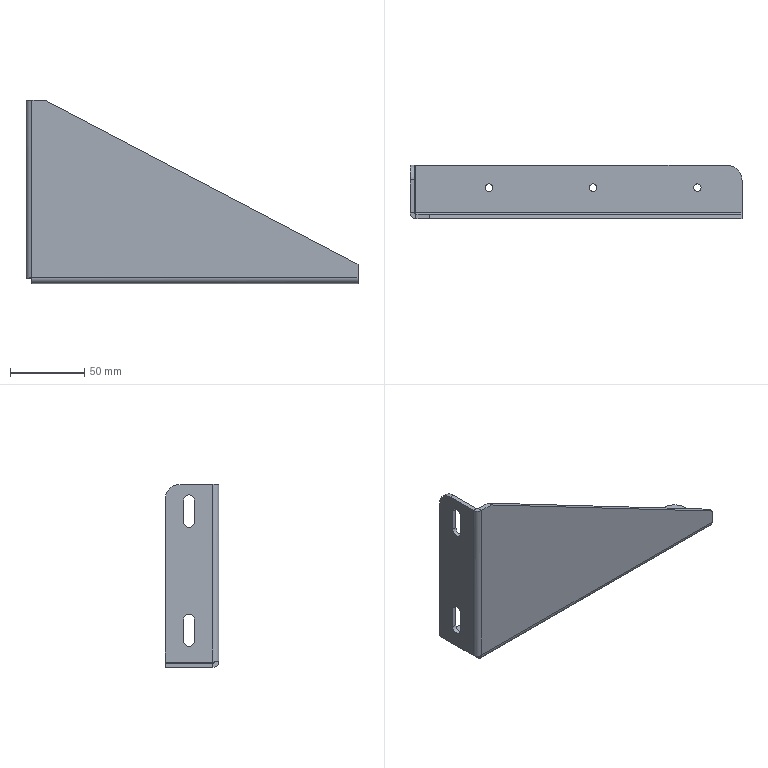Part | SolidWorks | features Cut 1, EdgeFlange 1, Fillet 1, FlatPattern 1, HoleWzd 1, LPattern 1, SMBaseFlange 1, SheetMetal 1 | 1 solid | 39 faces | box 223 x 36 x 123 mm | volume 78856 mm3 | plane 21 | cylinder 16 | spline 2 | commonest cylinder face diameters 5 x6 7 x4 2 x2 8 x2 20 x2
STEP:
#1=CARTESIAN_POINT('',(47.5,21.,-3.));
#2=VERTEX_POINT('',#1);
#3=CARTESIAN_POINT('',(52.5,21.,-3.));
#4=VERTEX_POINT('',#3);
#5=CARTESIAN_POINT('',(50.,21.,-3.));
#6=DIRECTION('',(0.,0.,1.));
#7=DIRECTION('',(1.,0.,0.));
#8=AXIS2_PLACEMENT_3D('',#5,#6,#7);
#9=CIRCLE('',#8,2.5);
#10=EDGE_CURVE('',#2,#4,#9,.T.);
#11=ORIENTED_EDGE('',*,*,#10,.F.);
#12=CARTESIAN_POINT('',(47.5,21.,0.));
#13=VERTEX_POINT('',#12);
#14=CARTESIAN_POINT('',(47.5,21.,0.));
#15=DIRECTION('',(0.,0.,1.));
#16=VECTOR('',#15,1000.);
#17=LINE('',#14,#16);
#18=EDGE_CURVE('',#2,#13,#17,.T.);
#19=ORIENTED_EDGE('',*,*,#18,.T.);
#20=CARTESIAN_POINT('',(52.5,21.,0.));
#21=VERTEX_POINT('',#20);
#22=CARTESIAN_POINT('',(50.,21.,0.));
#23=DIRECTION('',(0.,0.,1.));
#24=DIRECTION('',(1.,0.,0.));
#25=AXIS2_PLACEMENT_3D('',#22,#23,#24);
#26=CIRCLE('',#25,2.5);
#27=EDGE_CURVE('',#13,#21,#26,.T.);
#28=ORIENTED_EDGE('',*,*,#27,.T.);
#29=CARTESIAN_POINT('',(52.5,21.,0.));
#30=DIRECTION('',(0.,0.,1.));
#31=VECTOR('',#30,1000.);
#32=LINE('',#29,#31);
#33=EDGE_CURVE('',#4,#21,#32,.T.);
#34=ORIENTED_EDGE('',*,*,#33,.F.);
#35=EDGE_LOOP('',(#11,#19,#28,#34));
#36=FACE_OUTER_BOUND('',#35,.T.);
#37=CARTESIAN_POINT('',(50.,21.,0.));
#38=DIRECTION('',(0.,0.,1.));
#39=DIRECTION('',(1.,0.,0.));
#40=AXIS2_PLACEMENT_3D('',#37,#38,#39);
#41=CYLINDRICAL_SURFACE('',#40,2.5);
#42=ADVANCED_FACE('',(#36),#41,.F.);
#43=CARTESIAN_POINT('',(117.5,21.,-3.));
#44=VERTEX_POINT('',#43);
#45=CARTESIAN_POINT('',(122.5,21.,-3.));
#46=VERTEX_POINT('',#45);
#47=CARTESIAN_POINT('',(120.,21.,-3.));
#48=DIRECTION('',(0.,0.,1.));
#49=DIRECTION('',(1.,0.,0.));
#50=AXIS2_PLACEMENT_3D('',#47,#48,#49);
#51=CIRCLE('',#50,2.5);
#52=EDGE_CURVE('',#44,#46,#51,.T.);
#53=ORIENTED_EDGE('',*,*,#52,.F.);
#54=CARTESIAN_POINT('',(117.5,21.,0.));
#55=VERTEX_POINT('',#54);
#56=CARTESIAN_POINT('',(117.5,21.,0.));
#57=DIRECTION('',(0.,0.,1.));
#58=VECTOR('',#57,1000.);
#59=LINE('',#56,#58);
#60=EDGE_CURVE('',#44,#55,#59,.T.);
#61=ORIENTED_EDGE('',*,*,#60,.T.);
#62=CARTESIAN_POINT('',(122.5,21.,0.));
#63=VERTEX_POINT('',#62);
#64=CARTESIAN_POINT('',(120.,21.,0.));
#65=DIRECTION('',(0.,0.,1.));
#66=DIRECTION('',(1.,0.,0.));
#67=AXIS2_PLACEMENT_3D('',#64,#65,#66);
#68=CIRCLE('',#67,2.5);
#69=EDGE_CURVE('',#55,#63,#68,.T.);
#70=ORIENTED_EDGE('',*,*,#69,.T.);
#71=CARTESIAN_POINT('',(122.5,21.,0.));
#72=DIRECTION('',(0.,0.,1.));
#73=VECTOR('',#72,1000.);
#74=LINE('',#71,#73);
#75=EDGE_CURVE('',#46,#63,#74,.T.);
#76=ORIENTED_EDGE('',*,*,#75,.F.);
#77=EDGE_LOOP('',(#53,#61,#70,#76));
#78=FACE_OUTER_BOUND('',#77,.T.);
#79=CARTESIAN_POINT('',(120.,21.,0.));
#80=DIRECTION('',(0.,0.,1.));
#81=DIRECTION('',(1.,0.,0.));
#82=AXIS2_PLACEMENT_3D('',#79,#80,#81);
#83=CYLINDRICAL_SURFACE('',#82,2.5);
#84=ADVANCED_FACE('',(#78),#83,.F.);
#85=CARTESIAN_POINT('',(187.5,21.,-3.));
#86=VERTEX_POINT('',#85);
#87=CARTESIAN_POINT('',(192.5,21.,-3.));
#88=VERTEX_POINT('',#87);
#89=CARTESIAN_POINT('',(190.,21.,-3.));
#90=DIRECTION('',(0.,0.,1.));
#91=DIRECTION('',(1.,0.,0.));
#92=AXIS2_PLACEMENT_3D('',#89,#90,#91);
#93=CIRCLE('',#92,2.5);
#94=EDGE_CURVE('',#86,#88,#93,.T.);
#95=ORIENTED_EDGE('',*,*,#94,.F.);
#96=CARTESIAN_POINT('',(187.5,21.,0.));
#97=VERTEX_POINT('',#96);
#98=CARTESIAN_POINT('',(187.5,21.,0.));
#99=DIRECTION('',(0.,0.,1.));
#100=VECTOR('',#99,1000.);
#101=LINE('',#98,#100);
#102=EDGE_CURVE('',#86,#97,#101,.T.);
#103=ORIENTED_EDGE('',*,*,#102,.T.);
#104=CARTESIAN_POINT('',(192.5,21.,0.));
#105=VERTEX_POINT('',#104);
#106=CARTESIAN_POINT('',(190.,21.,0.));
#107=DIRECTION('',(0.,0.,1.));
#108=DIRECTION('',(1.,0.,0.));
#109=AXIS2_PLACEMENT_3D('',#106,#107,#108);
#110=CIRCLE('',#109,2.5);
#111=EDGE_CURVE('',#97,#105,#110,.T.);
#112=ORIENTED_EDGE('',*,*,#111,.T.);
#113=CARTESIAN_POINT('',(192.5,21.,0.));
#114=DIRECTION('',(0.,0.,1.));
#115=VECTOR('',#114,1000.);
#116=LINE('',#113,#115);
#117=EDGE_CURVE('',#88,#105,#116,.T.);
#118=ORIENTED_EDGE('',*,*,#117,.F.);
#119=EDGE_LOOP('',(#95,#103,#112,#118));
#120=FACE_OUTER_BOUND('',#119,.T.);
#121=CARTESIAN_POINT('',(190.,21.,0.));
#122=DIRECTION('',(0.,0.,1.));
#123=DIRECTION('',(1.,0.,0.));
#124=AXIS2_PLACEMENT_3D('',#121,#122,#123);
#125=CYLINDRICAL_SURFACE('',#124,2.5);
#126=ADVANCED_FACE('',(#120),#125,.F.);
#127=CARTESIAN_POINT('',(1.,3.,1.));
#128=VERTEX_POINT('',#127);
#129=CARTESIAN_POINT('',(220.,3.,1.));
#130=VERTEX_POINT('',#129);
#131=CARTESIAN_POINT('',(0.7071,3.,1.));
#132=DIRECTION('',(1.,0.,0.));
#133=VECTOR('',#132,1000.);
#134=LINE('',#131,#133);
#135=EDGE_CURVE('',#128,#130,#134,.T.);
#136=ORIENTED_EDGE('',*,*,#135,.F.);
#137=CARTESIAN_POINT('',(1.,3.,120.));
#138=VERTEX_POINT('',#137);
#139=CARTESIAN_POINT('',(1.,3.,120.));
#140=DIRECTION('',(0.,0.,-1.));
#141=VECTOR('',#140,1000.);
#142=LINE('',#139,#141);
#143=EDGE_CURVE('',#138,#128,#142,.T.);
#144=ORIENTED_EDGE('',*,*,#143,.F.);
#145=CARTESIAN_POINT('',(10.,3.,120.));
#146=VERTEX_POINT('',#145);
#147=CARTESIAN_POINT('',(10.,3.,120.));
#148=DIRECTION('',(1.,0.,0.));
#149=VECTOR('',#148,1000.);
#150=LINE('',#147,#149);
#151=EDGE_CURVE('',#138,#146,#150,.T.);
#152=ORIENTED_EDGE('',*,*,#151,.T.);
#153=CARTESIAN_POINT('',(220.,3.,10.));
#154=VERTEX_POINT('',#153);
#155=CARTESIAN_POINT('',(220.,3.,10.));
#156=DIRECTION('',(0.8858,0.,-0.464));
#157=VECTOR('',#156,1000.);
#158=LINE('',#155,#157);
#159=EDGE_CURVE('',#146,#154,#158,.T.);
#160=ORIENTED_EDGE('',*,*,#159,.T.);
#161=CARTESIAN_POINT('',(220.,3.,0.));
#162=DIRECTION('',(0.,0.,-1.));
#163=VECTOR('',#162,1000.);
#164=LINE('',#161,#163);
#165=EDGE_CURVE('',#154,#130,#164,.T.);
#166=ORIENTED_EDGE('',*,*,#165,.T.);
#167=EDGE_LOOP('',(#136,#144,#152,#160,#166));
#168=FACE_OUTER_BOUND('',#167,.T.);
#169=CARTESIAN_POINT('',(0.,3.,120.));
#170=DIRECTION('',(0.,-1.,0.));
#171=DIRECTION('',(0.,0.,-1.));
#172=AXIS2_PLACEMENT_3D('',#169,#170,#171);
#173=PLANE('',#172);
#174=ADVANCED_FACE('',(#168),#173,.F.);
#175=CARTESIAN_POINT('',(1.,0.,120.));
#176=VERTEX_POINT('',#175);
#177=CARTESIAN_POINT('',(1.,0.,1.));
#178=VERTEX_POINT('',#177);
#179=CARTESIAN_POINT('',(1.,0.,120.));
#180=DIRECTION('',(0.,0.,-1.));
#181=VECTOR('',#180,1000.);
#182=LINE('',#179,#181);
#183=EDGE_CURVE('',#176,#178,#182,.T.);
#184=ORIENTED_EDGE('',*,*,#183,.T.);
#185=CARTESIAN_POINT('',(220.,0.,1.));
#186=VERTEX_POINT('',#185);
#187=CARTESIAN_POINT('',(0.7071,0.,1.));
#188=DIRECTION('',(1.,0.,0.));
#189=VECTOR('',#188,1000.);
#190=LINE('',#187,#189);
#191=EDGE_CURVE('',#178,#186,#190,.T.);
#192=ORIENTED_EDGE('',*,*,#191,.T.);
#193=CARTESIAN_POINT('',(220.,0.,10.));
#194=VERTEX_POINT('',#193);
#195=CARTESIAN_POINT('',(220.,0.,0.));
#196=DIRECTION('',(0.,0.,-1.));
#197=VECTOR('',#196,1000.);
#198=LINE('',#195,#197);
#199=EDGE_CURVE('',#194,#186,#198,.T.);
#200=ORIENTED_EDGE('',*,*,#199,.F.);
#201=CARTESIAN_POINT('',(10.,0.,120.));
#202=VERTEX_POINT('',#201);
#203=CARTESIAN_POINT('',(220.,0.,10.));
#204=DIRECTION('',(0.8858,0.,-0.464));
#205=VECTOR('',#204,1000.);
#206=LINE('',#203,#205);
#207=EDGE_CURVE('',#202,#194,#206,.T.);
#208=ORIENTED_EDGE('',*,*,#207,.F.);
#209=CARTESIAN_POINT('',(10.,0.,120.));
#210=DIRECTION('',(1.,0.,0.));
#211=VECTOR('',#210,1000.);
#212=LINE('',#209,#211);
#213=EDGE_CURVE('',#176,#202,#212,.T.);
#214=ORIENTED_EDGE('',*,*,#213,.F.);
#215=EDGE_LOOP('',(#184,#192,#200,#208,#214));
#216=FACE_OUTER_BOUND('',#215,.T.);
#217=CARTESIAN_POINT('',(0.,0.,120.));
#218=DIRECTION('',(0.,-1.,0.));
#219=DIRECTION('',(0.,0.,-1.));
#220=AXIS2_PLACEMENT_3D('',#217,#218,#219);
#221=PLANE('',#220);
#222=ADVANCED_FACE('',(#216),#221,.T.);
#223=CARTESIAN_POINT('',(220.,3.,1.));
#224=DIRECTION('',(0.,-1.,0.));
#225=VECTOR('',#224,1000.);
#226=LINE('',#223,#225);
#227=EDGE_CURVE('',#130,#186,#226,.T.);
#228=ORIENTED_EDGE('',*,*,#227,.F.);
#229=ORIENTED_EDGE('',*,*,#165,.F.);
#230=CARTESIAN_POINT('',(220.,3.,10.));
#231=DIRECTION('',(0.,-1.,0.));
#232=VECTOR('',#231,1000.);
#233=LINE('',#230,#232);
#234=EDGE_CURVE('',#154,#194,#233,.T.);
#235=ORIENTED_EDGE('',*,*,#234,.T.);
#236=ORIENTED_EDGE('',*,*,#199,.T.);
#237=EDGE_LOOP('',(#228,#229,#235,#236));
#238=FACE_OUTER_BOUND('',#237,.T.);
#239=CARTESIAN_POINT('',(220.,3.,0.));
#240=DIRECTION('',(-1.,0.,0.));
#241=DIRECTION('',(0.,0.,1.));
#242=AXIS2_PLACEMENT_3D('',#239,#240,#241);
#243=PLANE('',#242);
#244=ADVANCED_FACE('',(#238),#243,.F.);
#245=CARTESIAN_POINT('',(1.,3.,120.));
#246=DIRECTION('',(0.,-1.,0.));
#247=VECTOR('',#246,1000.);
#248=LINE('',#245,#247);
#249=EDGE_CURVE('',#138,#176,#248,.T.);
#250=ORIENTED_EDGE('',*,*,#249,.T.);
#251=ORIENTED_EDGE('',*,*,#213,.T.);
#252=CARTESIAN_POINT('',(10.,3.,120.));
#253=DIRECTION('',(0.,-1.,0.));
#254=VECTOR('',#253,1000.);
#255=LINE('',#252,#254);
#256=EDGE_CURVE('',#146,#202,#255,.T.);
#257=ORIENTED_EDGE('',*,*,#256,.F.);
#258=ORIENTED_EDGE('',*,*,#151,.F.);
#259=EDGE_LOOP('',(#250,#251,#257,#258));
#260=FACE_OUTER_BOUND('',#259,.T.);
#261=CARTESIAN_POINT('',(10.,3.,120.));
#262=DIRECTION('',(0.,0.,-1.));
#263=DIRECTION('',(-1.,0.,0.));
#264=AXIS2_PLACEMENT_3D('',#261,#262,#263);
#265=PLANE('',#264);
#266=ADVANCED_FACE('',(#260),#265,.F.);
#267=ORIENTED_EDGE('',*,*,#207,.T.);
#268=ORIENTED_EDGE('',*,*,#234,.F.);
#269=ORIENTED_EDGE('',*,*,#159,.F.);
#270=ORIENTED_EDGE('',*,*,#256,.T.);
#271=EDGE_LOOP('',(#267,#268,#269,#270));
#272=FACE_OUTER_BOUND('',#271,.T.);
#273=CARTESIAN_POINT('',(220.,3.,10.));
#274=DIRECTION('',(-0.464,0.,-0.8858));
#275=DIRECTION('',(-0.8858,0.,0.464));
#276=AXIS2_PLACEMENT_3D('',#273,#274,#275);
#277=PLANE('',#276);
#278=ADVANCED_FACE('',(#272),#277,.F.);
#279=CARTESIAN_POINT('',(-3.,4.,0.7071));
#280=VERTEX_POINT('',#279);
#281=CARTESIAN_POINT('',(0.,4.,0.7071));
#282=VERTEX_POINT('',#281);
#283=CARTESIAN_POINT('',(0.,4.,0.7071));
#284=DIRECTION('',(1.,0.,0.));
#285=VECTOR('',#284,1000.);
#286=LINE('',#283,#285);
#287=EDGE_CURVE('',#280,#282,#286,.T.);
#288=ORIENTED_EDGE('',*,*,#287,.T.);
#289=CARTESIAN_POINT('',(1.,3.,1.));
#290=CARTESIAN_POINT('',(0.7382,3.,0.9512));
#291=CARTESIAN_POINT('',(0.478,3.108,0.9024));
#292=CARTESIAN_POINT('',(0.1078,3.478,0.8047));
#293=CARTESIAN_POINT('',(0.,3.738,0.7559));
#294=CARTESIAN_POINT('',(0.,4.,0.7071));
#295=B_SPLINE_CURVE_WITH_KNOTS('',3,(#289,#290,#291,#292,#293,#294),.UNSPECIFIED.,.F.,.F.,(4,2,4),(0.,0.5,1.),.UNSPECIFIED.);
#296=EDGE_CURVE('',#128,#282,#295,.T.);
#297=ORIENTED_EDGE('',*,*,#296,.F.);
#298=CARTESIAN_POINT('',(1.,3.,1.));
#299=DIRECTION('',(0.,-1.,0.));
#300=VECTOR('',#299,1000.);
#301=LINE('',#298,#300);
#302=EDGE_CURVE('',#128,#178,#301,.T.);
#303=ORIENTED_EDGE('',*,*,#302,.T.);
#304=CARTESIAN_POINT('',(1.,0.,1.));
#305=CARTESIAN_POINT('',(0.4764,0.,0.9756));
#306=CARTESIAN_POINT('',(-0.04699,0.1041,0.9512));
#307=CARTESIAN_POINT('',(-1.014,0.5049,0.9024));
#308=CARTESIAN_POINT('',(-1.458,0.8013,0.878));
#309=CARTESIAN_POINT('',(-2.199,1.542,0.8291));
#310=CARTESIAN_POINT('',(-2.495,1.986,0.8047));
#311=CARTESIAN_POINT('',(-2.896,2.953,0.7559));
#312=CARTESIAN_POINT('',(-3.,3.476,0.7315));
#313=CARTESIAN_POINT('',(-3.,4.,0.7071));
#314=B_SPLINE_CURVE_WITH_KNOTS('',3,(#304,#305,#306,#307,#308,#309,#310,#311,#312,#313),.UNSPECIFIED.,.F.,.F.,(4,2,2,2,4),(0.,0.25,0.5,0.75,1.),.UNSPECIFIED.);
#315=EDGE_CURVE('',#178,#280,#314,.T.);
#316=ORIENTED_EDGE('',*,*,#315,.T.);
#317=EDGE_LOOP('',(#288,#297,#303,#316));
#318=FACE_OUTER_BOUND('',#317,.T.);
#319=CARTESIAN_POINT('',(1.,-0.03,1.));
#320=CARTESIAN_POINT('',(0.4724,-0.03,0.9756));
#321=CARTESIAN_POINT('',(-0.05484,0.07489,0.9512));
#322=CARTESIAN_POINT('',(-1.03,0.4786,0.9024));
#323=CARTESIAN_POINT('',(-1.477,0.7773,0.878));
#324=CARTESIAN_POINT('',(-2.223,1.523,0.8291));
#325=CARTESIAN_POINT('',(-2.521,1.97,0.8047));
#326=CARTESIAN_POINT('',(-2.925,2.945,0.7559));
#327=CARTESIAN_POINT('',(-3.03,3.472,0.7315));
#328=CARTESIAN_POINT('',(-3.03,4.,0.7071));
#329=CARTESIAN_POINT('',(1.,0.,1.));
#330=CARTESIAN_POINT('',(0.4763,0.,0.9756));
#331=CARTESIAN_POINT('',(-0.04699,0.1041,0.9512));
#332=CARTESIAN_POINT('',(-1.014,0.5049,0.9024));
#333=CARTESIAN_POINT('',(-1.458,0.8013,0.878));
#334=CARTESIAN_POINT('',(-2.199,1.542,0.8291));
#335=CARTESIAN_POINT('',(-2.495,1.986,0.8047));
#336=CARTESIAN_POINT('',(-2.896,2.953,0.7559));
#337=CARTESIAN_POINT('',(-3.,3.476,0.7315));
#338=CARTESIAN_POINT('',(-3.,4.,0.7071));
#339=CARTESIAN_POINT('',(1.,3.,1.));
#340=CARTESIAN_POINT('',(0.8691,3.,0.9756));
#341=CARTESIAN_POINT('',(0.7383,3.026,0.9512));
#342=CARTESIAN_POINT('',(0.4964,3.126,0.9024));
#343=CARTESIAN_POINT('',(0.3855,3.2,0.878));
#344=CARTESIAN_POINT('',(0.2003,3.385,0.8291));
#345=CARTESIAN_POINT('',(0.1262,3.496,0.8047));
#346=CARTESIAN_POINT('',(0.02603,3.738,0.7559));
#347=CARTESIAN_POINT('',(0.,3.869,0.7315));
#348=CARTESIAN_POINT('',(0.,4.,0.7071));
#349=CARTESIAN_POINT('',(1.,3.03,1.));
#350=CARTESIAN_POINT('',(0.873,3.03,0.9756));
#351=CARTESIAN_POINT('',(0.7462,3.056,0.9512));
#352=CARTESIAN_POINT('',(0.5116,3.153,0.9024));
#353=CARTESIAN_POINT('',(0.4041,3.225,0.878));
#354=CARTESIAN_POINT('',(0.2246,3.404,0.8291));
#355=CARTESIAN_POINT('',(0.1527,3.512,0.8047));
#356=CARTESIAN_POINT('',(0.05554,3.746,0.7559));
#357=CARTESIAN_POINT('',(0.0303,3.873,0.7315));
#358=CARTESIAN_POINT('',(0.0303,4.,0.7071));
#359=B_SPLINE_SURFACE_WITH_KNOTS('',1,3,((#319,#320,#321,#322,#323,#324,#325,#326,#327,#328),(#329,#330,#331,#332,#333,#334,#335,#336,#337,#338),(#339,#340,#341,#342,#343,#344,#345,#346,#347,#348),(#349,#350,#351,#352,#353,#354,#355,#356,#357,#358)),.UNSPECIFIED.,.F.,.F.,.F.,(2,1,1,2),(4,2,2,2,4),(-0.01,0.,1.,1.01),(0.,0.25,0.5,0.75,1.),.UNSPECIFIED.);
#360=ADVANCED_FACE('',(#318),#359,.F.);
#361=ORIENTED_EDGE('',*,*,#183,.F.);
#362=CARTESIAN_POINT('',(-3.,4.,120.));
#363=VERTEX_POINT('',#362);
#364=CARTESIAN_POINT('',(1.,4.,120.));
#365=DIRECTION('',(0.,0.,1.));
#366=DIRECTION('',(1.,0.,0.));
#367=AXIS2_PLACEMENT_3D('',#364,#365,#366);
#368=CIRCLE('',#367,4.);
#369=EDGE_CURVE('',#363,#176,#368,.T.);
#370=ORIENTED_EDGE('',*,*,#369,.F.);
#371=CARTESIAN_POINT('',(-3.,4.,0.));
#372=DIRECTION('',(0.,0.,-1.));
#373=VECTOR('',#372,1000.);
#374=LINE('',#371,#373);
#375=EDGE_CURVE('',#363,#280,#374,.T.);
#376=ORIENTED_EDGE('',*,*,#375,.T.);
#377=ORIENTED_EDGE('',*,*,#315,.F.);
#378=EDGE_LOOP('',(#361,#370,#376,#377));
#379=FACE_OUTER_BOUND('',#378,.T.);
#380=CARTESIAN_POINT('',(1.,4.,120.));
#381=DIRECTION('',(0.,0.,1.));
#382=DIRECTION('',(-1.,0.,0.));
#383=AXIS2_PLACEMENT_3D('',#380,#381,#382);
#384=CYLINDRICAL_SURFACE('',#383,4.);
#385=ADVANCED_FACE('',(#379),#384,.T.);
#386=CARTESIAN_POINT('',(0.,4.,120.));
#387=VERTEX_POINT('',#386);
#388=CARTESIAN_POINT('',(1.,4.,120.));
#389=DIRECTION('',(0.,0.,1.));
#390=DIRECTION('',(1.,0.,0.));
#391=AXIS2_PLACEMENT_3D('',#388,#389,#390);
#392=CIRCLE('',#391,1.);
#393=EDGE_CURVE('',#387,#138,#392,.T.);
#394=ORIENTED_EDGE('',*,*,#393,.F.);
#395=CARTESIAN_POINT('',(0.,4.,120.));
#396=DIRECTION('',(-1.,0.,0.));
#397=VECTOR('',#396,1000.);
#398=LINE('',#395,#397);
#399=EDGE_CURVE('',#387,#363,#398,.T.);
#400=ORIENTED_EDGE('',*,*,#399,.T.);
#401=ORIENTED_EDGE('',*,*,#369,.T.);
#402=ORIENTED_EDGE('',*,*,#249,.F.);
#403=EDGE_LOOP('',(#394,#400,#401,#402));
#404=FACE_OUTER_BOUND('',#403,.T.);
#405=CARTESIAN_POINT('',(1.,4.,120.));
#406=DIRECTION('',(0.,0.,-1.));
#407=DIRECTION('',(-1.,0.,0.));
#408=AXIS2_PLACEMENT_3D('',#405,#406,#407);
#409=PLANE('',#408);
#410=ADVANCED_FACE('',(#404),#409,.F.);
#411=ORIENTED_EDGE('',*,*,#143,.T.);
#412=ORIENTED_EDGE('',*,*,#296,.T.);
#413=CARTESIAN_POINT('',(0.,4.,0.));
#414=DIRECTION('',(0.,0.,1.));
#415=VECTOR('',#414,1000.);
#416=LINE('',#413,#415);
#417=EDGE_CURVE('',#282,#387,#416,.T.);
#418=ORIENTED_EDGE('',*,*,#417,.T.);
#419=ORIENTED_EDGE('',*,*,#393,.T.);
#420=EDGE_LOOP('',(#411,#412,#418,#419));
#421=FACE_OUTER_BOUND('',#420,.T.);
#422=CARTESIAN_POINT('',(1.,4.,120.));
#423=DIRECTION('',(0.,0.,1.));
#424=DIRECTION('',(-1.,0.,0.));
#425=AXIS2_PLACEMENT_3D('',#422,#423,#424);
#426=CYLINDRICAL_SURFACE('',#425,1.);
#427=ADVANCED_FACE('',(#421),#426,.F.);
#428=CARTESIAN_POINT('',(-3.,36.,0.7071));
#429=VERTEX_POINT('',#428);
#430=CARTESIAN_POINT('',(-3.,36.,0.7071));
#431=DIRECTION('',(0.,1.,0.));
#432=VECTOR('',#431,1000.);
#433=LINE('',#430,#432);
#434=EDGE_CURVE('',#280,#429,#433,.T.);
#435=ORIENTED_EDGE('',*,*,#434,.T.);
#436=CARTESIAN_POINT('',(0.,36.,0.7071));
#437=VERTEX_POINT('',#436);
#438=CARTESIAN_POINT('',(-3.,36.,0.7071));
#439=DIRECTION('',(1.,0.,0.));
#440=VECTOR('',#439,1000.);
#441=LINE('',#438,#440);
#442=EDGE_CURVE('',#429,#437,#441,.T.);
#443=ORIENTED_EDGE('',*,*,#442,.T.);
#444=CARTESIAN_POINT('',(0.,3.,0.7071));
#445=DIRECTION('',(0.,1.,0.));
#446=VECTOR('',#445,1000.);
#447=LINE('',#444,#446);
#448=EDGE_CURVE('',#282,#437,#447,.T.);
#449=ORIENTED_EDGE('',*,*,#448,.F.);
#450=ORIENTED_EDGE('',*,*,#287,.F.);
#451=EDGE_LOOP('',(#435,#443,#449,#450));
#452=FACE_OUTER_BOUND('',#451,.T.);
#453=CARTESIAN_POINT('',(0.,3.,0.7071));
#454=DIRECTION('',(0.,0.,-1.));
#455=DIRECTION('',(-1.,0.,0.));
#456=AXIS2_PLACEMENT_3D('',#453,#454,#455);
#457=PLANE('',#456);
#458=ADVANCED_FACE('',(#452),#457,.T.);
#459=CARTESIAN_POINT('',(-3.,23.5,14.5));
#460=VERTEX_POINT('',#459);
#461=CARTESIAN_POINT('',(-3.,23.5,29.5));
#462=VERTEX_POINT('',#461);
#463=CARTESIAN_POINT('',(-3.,23.5,0.));
#464=DIRECTION('',(0.,0.,1.));
#465=VECTOR('',#464,1000.);
#466=LINE('',#463,#465);
#467=EDGE_CURVE('',#460,#462,#466,.T.);
#468=ORIENTED_EDGE('',*,*,#467,.T.);
#469=CARTESIAN_POINT('',(-3.,16.5,29.5));
#470=VERTEX_POINT('',#469);
#471=CARTESIAN_POINT('',(-3.,20.,29.5));
#472=DIRECTION('',(1.,0.,0.));
#473=DIRECTION('',(0.,1.,0.));
#474=AXIS2_PLACEMENT_3D('',#471,#472,#473);
#475=CIRCLE('',#474,3.5);
#476=EDGE_CURVE('',#462,#470,#475,.T.);
#477=ORIENTED_EDGE('',*,*,#476,.T.);
#478=CARTESIAN_POINT('',(-3.,16.5,14.5));
#479=VERTEX_POINT('',#478);
#480=CARTESIAN_POINT('',(-3.,16.5,0.));
#481=DIRECTION('',(0.,0.,-1.));
#482=VECTOR('',#481,1000.);
#483=LINE('',#480,#482);
#484=EDGE_CURVE('',#470,#479,#483,.T.);
#485=ORIENTED_EDGE('',*,*,#484,.T.);
#486=CARTESIAN_POINT('',(-3.,20.,14.5));
#487=DIRECTION('',(1.,0.,0.));
#488=DIRECTION('',(0.,1.,0.));
#489=AXIS2_PLACEMENT_3D('',#486,#487,#488);
#490=CIRCLE('',#489,3.5);
#491=EDGE_CURVE('',#479,#460,#490,.T.);
#492=ORIENTED_EDGE('',*,*,#491,.T.);
#493=EDGE_LOOP('',(#468,#477,#485,#492));
#494=FACE_BOUND('',#493,.T.);
#495=CARTESIAN_POINT('',(-3.,23.5,94.5));
#496=VERTEX_POINT('',#495);
#497=CARTESIAN_POINT('',(-3.,23.5,109.5));
#498=VERTEX_POINT('',#497);
#499=CARTESIAN_POINT('',(-3.,23.5,0.));
#500=DIRECTION('',(0.,0.,1.));
#501=VECTOR('',#500,1000.);
#502=LINE('',#499,#501);
#503=EDGE_CURVE('',#496,#498,#502,.T.);
#504=ORIENTED_EDGE('',*,*,#503,.T.);
#505=CARTESIAN_POINT('',(-3.,16.5,109.5));
#506=VERTEX_POINT('',#505);
#507=CARTESIAN_POINT('',(-3.,20.,109.5));
#508=DIRECTION('',(1.,0.,0.));
#509=DIRECTION('',(0.,1.,0.));
#510=AXIS2_PLACEMENT_3D('',#507,#508,#509);
#511=CIRCLE('',#510,3.5);
#512=EDGE_CURVE('',#498,#506,#511,.T.);
#513=ORIENTED_EDGE('',*,*,#512,.T.);
#514=CARTESIAN_POINT('',(-3.,16.5,94.5));
#515=VERTEX_POINT('',#514);
#516=CARTESIAN_POINT('',(-3.,16.5,0.));
#517=DIRECTION('',(0.,0.,-1.));
#518=VECTOR('',#517,1000.);
#519=LINE('',#516,#518);
#520=EDGE_CURVE('',#506,#515,#519,.T.);
#521=ORIENTED_EDGE('',*,*,#520,.T.);
#522=CARTESIAN_POINT('',(-3.,20.,94.5));
#523=DIRECTION('',(1.,0.,0.));
#524=DIRECTION('',(0.,1.,0.));
#525=AXIS2_PLACEMENT_3D('',#522,#523,#524);
#526=CIRCLE('',#525,3.5);
#527=EDGE_CURVE('',#515,#496,#526,.T.);
#528=ORIENTED_EDGE('',*,*,#527,.T.);
#529=EDGE_LOOP('',(#504,#513,#521,#528));
#530=FACE_BOUND('',#529,.T.);
#531=CARTESIAN_POINT('',(-3.,26.,120.));
#532=VERTEX_POINT('',#531);
#533=CARTESIAN_POINT('',(-3.,36.,120.));
#534=DIRECTION('',(0.,1.,0.));
#535=VECTOR('',#534,1000.);
#536=LINE('',#533,#535);
#537=EDGE_CURVE('',#363,#532,#536,.T.);
#538=ORIENTED_EDGE('',*,*,#537,.T.);
#539=CARTESIAN_POINT('',(-3.,36.,110.));
#540=VERTEX_POINT('',#539);
#541=CARTESIAN_POINT('',(-3.,26.,110.));
#542=DIRECTION('',(-1.,0.,0.));
#543=DIRECTION('',(0.,1.,0.));
#544=AXIS2_PLACEMENT_3D('',#541,#542,#543);
#545=CIRCLE('',#544,10.);
#546=EDGE_CURVE('',#532,#540,#545,.T.);
#547=ORIENTED_EDGE('',*,*,#546,.T.);
#548=CARTESIAN_POINT('',(-3.,36.,0.));
#549=DIRECTION('',(0.,0.,-1.));
#550=VECTOR('',#549,1000.);
#551=LINE('',#548,#550);
#552=EDGE_CURVE('',#540,#429,#551,.T.);
#553=ORIENTED_EDGE('',*,*,#552,.T.);
#554=ORIENTED_EDGE('',*,*,#434,.F.);
#555=ORIENTED_EDGE('',*,*,#375,.F.);
#556=EDGE_LOOP('',(#538,#547,#553,#554,#555));
#557=FACE_OUTER_BOUND('',#556,.T.);
#558=CARTESIAN_POINT('',(-3.,36.,0.));
#559=DIRECTION('',(1.,0.,0.));
#560=DIRECTION('',(0.,1.,0.));
#561=AXIS2_PLACEMENT_3D('',#558,#559,#560);
#562=PLANE('',#561);
#563=ADVANCED_FACE('',(#494,#530,#557),#562,.F.);
#564=CARTESIAN_POINT('',(0.,23.5,29.5));
#565=VERTEX_POINT('',#564);
#566=CARTESIAN_POINT('',(0.,16.5,29.5));
#567=VERTEX_POINT('',#566);
#568=CARTESIAN_POINT('',(0.,20.,29.5));
#569=DIRECTION('',(1.,0.,0.));
#570=DIRECTION('',(0.,1.,0.));
#571=AXIS2_PLACEMENT_3D('',#568,#569,#570);
#572=CIRCLE('',#571,3.5);
#573=EDGE_CURVE('',#565,#567,#572,.T.);
#574=ORIENTED_EDGE('',*,*,#573,.F.);
#575=CARTESIAN_POINT('',(0.,23.5,14.5));
#576=VERTEX_POINT('',#575);
#577=CARTESIAN_POINT('',(0.,23.5,29.5));
#578=DIRECTION('',(0.,0.,1.));
#579=VECTOR('',#578,1000.);
#580=LINE('',#577,#579);
#581=EDGE_CURVE('',#576,#565,#580,.T.);
#582=ORIENTED_EDGE('',*,*,#581,.F.);
#583=CARTESIAN_POINT('',(0.,16.5,14.5));
#584=VERTEX_POINT('',#583);
#585=CARTESIAN_POINT('',(0.,20.,14.5));
#586=DIRECTION('',(1.,0.,0.));
#587=DIRECTION('',(0.,-1.,0.));
#588=AXIS2_PLACEMENT_3D('',#585,#586,#587);
#589=CIRCLE('',#588,3.5);
#590=EDGE_CURVE('',#584,#576,#589,.T.);
#591=ORIENTED_EDGE('',*,*,#590,.F.);
#592=CARTESIAN_POINT('',(0.,16.5,29.5));
#593=DIRECTION('',(0.,0.,-1.));
#594=VECTOR('',#593,1000.);
#595=LINE('',#592,#594);
#596=EDGE_CURVE('',#567,#584,#595,.T.);
#597=ORIENTED_EDGE('',*,*,#596,.F.);
#598=EDGE_LOOP('',(#574,#582,#591,#597));
#599=FACE_BOUND('',#598,.T.);
#600=CARTESIAN_POINT('',(0.,23.5,109.5));
#601=VERTEX_POINT('',#600);
#602=CARTESIAN_POINT('',(0.,16.5,109.5));
#603=VERTEX_POINT('',#602);
#604=CARTESIAN_POINT('',(0.,20.,109.5));
#605=DIRECTION('',(1.,0.,0.));
#606=DIRECTION('',(0.,1.,0.));
#607=AXIS2_PLACEMENT_3D('',#604,#605,#606);
#608=CIRCLE('',#607,3.5);
#609=EDGE_CURVE('',#601,#603,#608,.T.);
#610=ORIENTED_EDGE('',*,*,#609,.F.);
#611=CARTESIAN_POINT('',(0.,23.5,94.5));
#612=VERTEX_POINT('',#611);
#613=CARTESIAN_POINT('',(0.,23.5,109.5));
#614=DIRECTION('',(0.,0.,1.));
#615=VECTOR('',#614,1000.);
#616=LINE('',#613,#615);
#617=EDGE_CURVE('',#612,#601,#616,.T.);
#618=ORIENTED_EDGE('',*,*,#617,.F.);
#619=CARTESIAN_POINT('',(0.,16.5,94.5));
#620=VERTEX_POINT('',#619);
#621=CARTESIAN_POINT('',(0.,20.,94.5));
#622=DIRECTION('',(1.,0.,0.));
#623=DIRECTION('',(0.,-1.,0.));
#624=AXIS2_PLACEMENT_3D('',#621,#622,#623);
#625=CIRCLE('',#624,3.5);
#626=EDGE_CURVE('',#620,#612,#625,.T.);
#627=ORIENTED_EDGE('',*,*,#626,.F.);
#628=CARTESIAN_POINT('',(0.,16.5,109.5));
#629=DIRECTION('',(0.,0.,-1.));
#630=VECTOR('',#629,1000.);
#631=LINE('',#628,#630);
#632=EDGE_CURVE('',#603,#620,#631,.T.);
#633=ORIENTED_EDGE('',*,*,#632,.F.);
#634=EDGE_LOOP('',(#610,#618,#627,#633));
#635=FACE_BOUND('',#634,.T.);
#636=CARTESIAN_POINT('',(0.,36.,110.));
#637=VERTEX_POINT('',#636);
#638=CARTESIAN_POINT('',(0.,36.,0.));
#639=DIRECTION('',(0.,0.,-1.));
#640=VECTOR('',#639,1000.);
#641=LINE('',#638,#640);
#642=EDGE_CURVE('',#637,#437,#641,.T.);
#643=ORIENTED_EDGE('',*,*,#642,.F.);
#644=CARTESIAN_POINT('',(0.,26.,120.));
#645=VERTEX_POINT('',#644);
#646=CARTESIAN_POINT('',(0.,26.,110.));
#647=DIRECTION('',(1.,0.,0.));
#648=DIRECTION('',(0.,1.,0.));
#649=AXIS2_PLACEMENT_3D('',#646,#647,#648);
#650=CIRCLE('',#649,10.);
#651=EDGE_CURVE('',#637,#645,#650,.T.);
#652=ORIENTED_EDGE('',*,*,#651,.T.);
#653=CARTESIAN_POINT('',(0.,36.,120.));
#654=DIRECTION('',(0.,1.,0.));
#655=VECTOR('',#654,1000.);
#656=LINE('',#653,#655);
#657=EDGE_CURVE('',#387,#645,#656,.T.);
#658=ORIENTED_EDGE('',*,*,#657,.F.);
#659=ORIENTED_EDGE('',*,*,#417,.F.);
#660=ORIENTED_EDGE('',*,*,#448,.T.);
#661=EDGE_LOOP('',(#643,#652,#658,#659,#660));
#662=FACE_OUTER_BOUND('',#661,.T.);
#663=CARTESIAN_POINT('',(0.,36.,0.));
#664=DIRECTION('',(1.,0.,0.));
#665=DIRECTION('',(0.,1.,0.));
#666=AXIS2_PLACEMENT_3D('',#663,#664,#665);
#667=PLANE('',#666);
#668=ADVANCED_FACE('',(#599,#635,#662),#667,.T.);
#669=ORIENTED_EDGE('',*,*,#552,.F.);
#670=CARTESIAN_POINT('',(-3.,36.,110.));
#671=DIRECTION('',(1.,0.,0.));
#672=VECTOR('',#671,1000.);
#673=LINE('',#670,#672);
#674=EDGE_CURVE('',#540,#637,#673,.T.);
#675=ORIENTED_EDGE('',*,*,#674,.T.);
#676=ORIENTED_EDGE('',*,*,#642,.T.);
#677=ORIENTED_EDGE('',*,*,#442,.F.);
#678=EDGE_LOOP('',(#669,#675,#676,#677));
#679=FACE_OUTER_BOUND('',#678,.T.);
#680=CARTESIAN_POINT('',(-3.,36.,0.));
#681=DIRECTION('',(0.,-1.,0.));
#682=DIRECTION('',(1.,0.,0.));
#683=AXIS2_PLACEMENT_3D('',#680,#681,#682);
#684=PLANE('',#683);
#685=ADVANCED_FACE('',(#679),#684,.F.);
#686=ORIENTED_EDGE('',*,*,#657,.T.);
#687=CARTESIAN_POINT('',(-3.,26.,120.));
#688=DIRECTION('',(-1.,0.,0.));
#689=VECTOR('',#688,1000.);
#690=LINE('',#687,#689);
#691=EDGE_CURVE('',#645,#532,#690,.T.);
#692=ORIENTED_EDGE('',*,*,#691,.T.);
#693=ORIENTED_EDGE('',*,*,#537,.F.);
#694=ORIENTED_EDGE('',*,*,#399,.F.);
#695=EDGE_LOOP('',(#686,#692,#693,#694));
#696=FACE_OUTER_BOUND('',#695,.T.);
#697=CARTESIAN_POINT('',(-3.,36.,120.));
#698=DIRECTION('',(0.,0.,-1.));
#699=DIRECTION('',(0.,1.,0.));
#700=AXIS2_PLACEMENT_3D('',#697,#698,#699);
#701=PLANE('',#700);
#702=ADVANCED_FACE('',(#696),#701,.F.);
#703=CARTESIAN_POINT('',(220.,4.,0.));
#704=VERTEX_POINT('',#703);
#705=CARTESIAN_POINT('',(220.,4.,-3.));
#706=VERTEX_POINT('',#705);
#707=CARTESIAN_POINT('',(220.,4.,0.));
#708=DIRECTION('',(0.,0.,-1.));
#709=VECTOR('',#708,1000.);
#710=LINE('',#707,#709);
#711=EDGE_CURVE('',#704,#706,#710,.T.);
#712=ORIENTED_EDGE('',*,*,#711,.F.);
#713=CARTESIAN_POINT('',(220.,4.,1.));
#714=DIRECTION('',(1.,0.,0.));
#715=DIRECTION('',(0.,0.,1.));
#716=AXIS2_PLACEMENT_3D('',#713,#714,#715);
#717=CIRCLE('',#716,1.);
#718=EDGE_CURVE('',#130,#704,#717,.T.);
#719=ORIENTED_EDGE('',*,*,#718,.F.);
#720=ORIENTED_EDGE('',*,*,#227,.T.);
#721=CARTESIAN_POINT('',(220.,4.,1.));
#722=DIRECTION('',(1.,0.,0.));
#723=DIRECTION('',(0.,0.,1.));
#724=AXIS2_PLACEMENT_3D('',#721,#722,#723);
#725=CIRCLE('',#724,4.);
#726=EDGE_CURVE('',#186,#706,#725,.T.);
#727=ORIENTED_EDGE('',*,*,#726,.T.);
#728=EDGE_LOOP('',(#712,#719,#720,#727));
#729=FACE_OUTER_BOUND('',#728,.T.);
#730=CARTESIAN_POINT('',(220.,4.,1.));
#731=DIRECTION('',(1.,0.,0.));
#732=DIRECTION('',(0.,0.,-1.));
#733=AXIS2_PLACEMENT_3D('',#730,#731,#732);
#734=PLANE('',#733);
#735=ADVANCED_FACE('',(#729),#734,.T.);
#736=ORIENTED_EDGE('',*,*,#191,.F.);
#737=CARTESIAN_POINT('',(0.7071,4.,-3.));
#738=VERTEX_POINT('',#737);
#739=CARTESIAN_POINT('',(0.7071,4.,-3.));
#740=CARTESIAN_POINT('',(0.7315,3.476,-3.));
#741=CARTESIAN_POINT('',(0.7559,2.953,-2.896));
#742=CARTESIAN_POINT('',(0.8047,1.986,-2.495));
#743=CARTESIAN_POINT('',(0.8291,1.542,-2.199));
#744=CARTESIAN_POINT('',(0.878,0.8013,-1.458));
#745=CARTESIAN_POINT('',(0.9024,0.5049,-1.014));
#746=CARTESIAN_POINT('',(0.9512,0.1041,-0.04699));
#747=CARTESIAN_POINT('',(0.9756,0.,0.4764));
#748=CARTESIAN_POINT('',(1.,0.,1.));
#749=B_SPLINE_CURVE_WITH_KNOTS('',3,(#739,#740,#741,#742,#743,#744,#745,#746,#747,#748),.UNSPECIFIED.,.F.,.F.,(4,2,2,2,4),(0.,0.25,0.5,0.75,1.),.UNSPECIFIED.);
#750=EDGE_CURVE('',#738,#178,#749,.T.);
#751=ORIENTED_EDGE('',*,*,#750,.F.);
#752=CARTESIAN_POINT('',(220.,4.,-3.));
#753=DIRECTION('',(1.,0.,0.));
#754=VECTOR('',#753,1000.);
#755=LINE('',#752,#754);
#756=EDGE_CURVE('',#738,#706,#755,.T.);
#757=ORIENTED_EDGE('',*,*,#756,.T.);
#758=ORIENTED_EDGE('',*,*,#726,.F.);
#759=EDGE_LOOP('',(#736,#751,#757,#758));
#760=FACE_OUTER_BOUND('',#759,.T.);
#761=CARTESIAN_POINT('',(0.7071,4.,1.));
#762=DIRECTION('',(-1.,0.,0.));
#763=DIRECTION('',(0.,0.,-1.));
#764=AXIS2_PLACEMENT_3D('',#761,#762,#763);
#765=CYLINDRICAL_SURFACE('',#764,4.);
#766=ADVANCED_FACE('',(#760),#765,.T.);
#767=CARTESIAN_POINT('',(0.7071,4.,0.));
#768=VERTEX_POINT('',#767);
#769=CARTESIAN_POINT('',(0.7071,4.,0.));
#770=CARTESIAN_POINT('',(0.7559,3.738,0.));
#771=CARTESIAN_POINT('',(0.8047,3.478,0.1078));
#772=CARTESIAN_POINT('',(0.9024,3.108,0.478));
#773=CARTESIAN_POINT('',(0.9512,3.,0.7382));
#774=CARTESIAN_POINT('',(1.,3.,1.));
#775=B_SPLINE_CURVE_WITH_KNOTS('',3,(#769,#770,#771,#772,#773,#774),.UNSPECIFIED.,.F.,.F.,(4,2,4),(0.,0.5,1.),.UNSPECIFIED.);
#776=EDGE_CURVE('',#768,#128,#775,.T.);
#777=ORIENTED_EDGE('',*,*,#776,.F.);
#778=CARTESIAN_POINT('',(0.7071,4.,0.));
#779=DIRECTION('',(0.,0.,1.));
#780=VECTOR('',#779,1000.);
#781=LINE('',#778,#780);
#782=EDGE_CURVE('',#738,#768,#781,.T.);
#783=ORIENTED_EDGE('',*,*,#782,.F.);
#784=ORIENTED_EDGE('',*,*,#750,.T.);
#785=ORIENTED_EDGE('',*,*,#302,.F.);
#786=EDGE_LOOP('',(#777,#783,#784,#785));
#787=FACE_OUTER_BOUND('',#786,.T.);
#788=CARTESIAN_POINT('',(0.7071,4.,-3.03));
#789=CARTESIAN_POINT('',(0.7315,3.472,-3.03));
#790=CARTESIAN_POINT('',(0.7559,2.945,-2.925));
#791=CARTESIAN_POINT('',(0.8047,1.97,-2.521));
#792=CARTESIAN_POINT('',(0.8291,1.523,-2.223));
#793=CARTESIAN_POINT('',(0.878,0.7773,-1.477));
#794=CARTESIAN_POINT('',(0.9024,0.4786,-1.03));
#795=CARTESIAN_POINT('',(0.9512,0.07489,-0.05484));
#796=CARTESIAN_POINT('',(0.9756,-0.03,0.4724));
#797=CARTESIAN_POINT('',(1.,-0.03,1.));
#798=CARTESIAN_POINT('',(0.7071,4.,-3.));
#799=CARTESIAN_POINT('',(0.7315,3.476,-3.));
#800=CARTESIAN_POINT('',(0.7559,2.953,-2.896));
#801=CARTESIAN_POINT('',(0.8047,1.986,-2.495));
#802=CARTESIAN_POINT('',(0.8291,1.542,-2.199));
#803=CARTESIAN_POINT('',(0.878,0.8013,-1.458));
#804=CARTESIAN_POINT('',(0.9024,0.5049,-1.014));
#805=CARTESIAN_POINT('',(0.9512,0.1041,-0.04699));
#806=CARTESIAN_POINT('',(0.9756,0.,0.4763));
#807=CARTESIAN_POINT('',(1.,0.,1.));
#808=CARTESIAN_POINT('',(0.7071,4.,0.));
#809=CARTESIAN_POINT('',(0.7315,3.869,0.));
#810=CARTESIAN_POINT('',(0.7559,3.738,0.02603));
#811=CARTESIAN_POINT('',(0.8047,3.496,0.1262));
#812=CARTESIAN_POINT('',(0.8291,3.385,0.2003));
#813=CARTESIAN_POINT('',(0.878,3.2,0.3855));
#814=CARTESIAN_POINT('',(0.9024,3.126,0.4964));
#815=CARTESIAN_POINT('',(0.9512,3.026,0.7383));
#816=CARTESIAN_POINT('',(0.9756,3.,0.8691));
#817=CARTESIAN_POINT('',(1.,3.,1.));
#818=CARTESIAN_POINT('',(0.7071,4.,0.0303));
#819=CARTESIAN_POINT('',(0.7315,3.873,0.0303));
#820=CARTESIAN_POINT('',(0.7559,3.746,0.05554));
#821=CARTESIAN_POINT('',(0.8047,3.512,0.1527));
#822=CARTESIAN_POINT('',(0.8291,3.404,0.2246));
#823=CARTESIAN_POINT('',(0.878,3.225,0.4041));
#824=CARTESIAN_POINT('',(0.9024,3.153,0.5116));
#825=CARTESIAN_POINT('',(0.9512,3.056,0.7462));
#826=CARTESIAN_POINT('',(0.9756,3.03,0.873));
#827=CARTESIAN_POINT('',(1.,3.03,1.));
#828=B_SPLINE_SURFACE_WITH_KNOTS('',1,3,((#788,#789,#790,#791,#792,#793,#794,#795,#796,#797),(#798,#799,#800,#801,#802,#803,#804,#805,#806,#807),(#808,#809,#810,#811,#812,#813,#814,#815,#816,#817),(#818,#819,#820,#821,#822,#823,#824,#825,#826,#827)),.UNSPECIFIED.,.F.,.F.,.F.,(2,1,1,2),(4,2,2,2,4),(-0.01,0.,1.,1.01),(0.,0.25,0.5,0.75,1.),.UNSPECIFIED.);
#829=ADVANCED_FACE('',(#787),#828,.F.);
#830=ORIENTED_EDGE('',*,*,#135,.T.);
#831=ORIENTED_EDGE('',*,*,#718,.T.);
#832=CARTESIAN_POINT('',(220.,4.,0.));
#833=DIRECTION('',(-1.,0.,0.));
#834=VECTOR('',#833,1000.);
#835=LINE('',#832,#834);
#836=EDGE_CURVE('',#704,#768,#835,.T.);
#837=ORIENTED_EDGE('',*,*,#836,.T.);
#838=ORIENTED_EDGE('',*,*,#776,.T.);
#839=EDGE_LOOP('',(#830,#831,#837,#838));
#840=FACE_OUTER_BOUND('',#839,.T.);
#841=CARTESIAN_POINT('',(0.7071,4.,1.));
#842=DIRECTION('',(-1.,0.,0.));
#843=DIRECTION('',(0.,0.,-1.));
#844=AXIS2_PLACEMENT_3D('',#841,#842,#843);
#845=CYLINDRICAL_SURFACE('',#844,1.);
#846=ADVANCED_FACE('',(#840),#845,.F.);
#847=CARTESIAN_POINT('',(220.,26.,-3.));
#848=VERTEX_POINT('',#847);
#849=CARTESIAN_POINT('',(220.,3.,-3.));
#850=DIRECTION('',(0.,-1.,0.));
#851=VECTOR('',#850,1000.);
#852=LINE('',#849,#851);
#853=EDGE_CURVE('',#848,#706,#852,.T.);
#854=ORIENTED_EDGE('',*,*,#853,.F.);
#855=CARTESIAN_POINT('',(220.,26.,0.));
#856=VERTEX_POINT('',#855);
#857=CARTESIAN_POINT('',(220.,26.,-3.));
#858=DIRECTION('',(0.,0.,1.));
#859=VECTOR('',#858,1000.);
#860=LINE('',#857,#859);
#861=EDGE_CURVE('',#848,#856,#860,.T.);
#862=ORIENTED_EDGE('',*,*,#861,.T.);
#863=CARTESIAN_POINT('',(220.,3.,0.));
#864=DIRECTION('',(0.,-1.,0.));
#865=VECTOR('',#864,1000.);
#866=LINE('',#863,#865);
#867=EDGE_CURVE('',#856,#704,#866,.T.);
#868=ORIENTED_EDGE('',*,*,#867,.T.);
#869=ORIENTED_EDGE('',*,*,#711,.T.);
#870=EDGE_LOOP('',(#854,#862,#868,#869));
#871=FACE_OUTER_BOUND('',#870,.T.);
#872=CARTESIAN_POINT('',(220.,3.,-3.));
#873=DIRECTION('',(-1.,0.,0.));
#874=DIRECTION('',(0.,0.,1.));
#875=AXIS2_PLACEMENT_3D('',#872,#873,#874);
#876=PLANE('',#875);
#877=ADVANCED_FACE('',(#871),#876,.F.);
#878=CARTESIAN_POINT('',(50.,21.,-3.));
#879=DIRECTION('',(0.,0.,1.));
#880=DIRECTION('',(1.,0.,0.));
#881=AXIS2_PLACEMENT_3D('',#878,#879,#880);
#882=CIRCLE('',#881,2.5);
#883=EDGE_CURVE('',#4,#2,#882,.T.);
#884=ORIENTED_EDGE('',*,*,#883,.T.);
#885=ORIENTED_EDGE('',*,*,#10,.T.);
#886=EDGE_LOOP('',(#884,#885));
#887=FACE_BOUND('',#886,.T.);
#888=CARTESIAN_POINT('',(120.,21.,-3.));
#889=DIRECTION('',(0.,0.,1.));
#890=DIRECTION('',(1.,0.,0.));
#891=AXIS2_PLACEMENT_3D('',#888,#889,#890);
#892=CIRCLE('',#891,2.5);
#893=EDGE_CURVE('',#46,#44,#892,.T.);
#894=ORIENTED_EDGE('',*,*,#893,.T.);
#895=ORIENTED_EDGE('',*,*,#52,.T.);
#896=EDGE_LOOP('',(#894,#895));
#897=FACE_BOUND('',#896,.T.);
#898=CARTESIAN_POINT('',(190.,21.,-3.));
#899=DIRECTION('',(0.,0.,1.));
#900=DIRECTION('',(1.,0.,0.));
#901=AXIS2_PLACEMENT_3D('',#898,#899,#900);
#902=CIRCLE('',#901,2.5);
#903=EDGE_CURVE('',#88,#86,#902,.T.);
#904=ORIENTED_EDGE('',*,*,#903,.T.);
#905=ORIENTED_EDGE('',*,*,#94,.T.);
#906=EDGE_LOOP('',(#904,#905));
#907=FACE_BOUND('',#906,.T.);
#908=CARTESIAN_POINT('',(0.7071,36.,-3.));
#909=VERTEX_POINT('',#908);
#910=CARTESIAN_POINT('',(210.,36.,-3.));
#911=VERTEX_POINT('',#910);
#912=CARTESIAN_POINT('',(220.,36.,-3.));
#913=DIRECTION('',(1.,0.,0.));
#914=VECTOR('',#913,1000.);
#915=LINE('',#912,#914);
#916=EDGE_CURVE('',#909,#911,#915,.T.);
#917=ORIENTED_EDGE('',*,*,#916,.T.);
#918=CARTESIAN_POINT('',(210.,26.,-3.));
#919=DIRECTION('',(0.,0.,-1.));
#920=DIRECTION('',(0.,-1.,0.));
#921=AXIS2_PLACEMENT_3D('',#918,#919,#920);
#922=CIRCLE('',#921,10.);
#923=EDGE_CURVE('',#911,#848,#922,.T.);
#924=ORIENTED_EDGE('',*,*,#923,.T.);
#925=ORIENTED_EDGE('',*,*,#853,.T.);
#926=ORIENTED_EDGE('',*,*,#756,.F.);
#927=CARTESIAN_POINT('',(0.7071,36.,-3.));
#928=DIRECTION('',(0.,1.,0.));
#929=VECTOR('',#928,1000.);
#930=LINE('',#927,#929);
#931=EDGE_CURVE('',#738,#909,#930,.T.);
#932=ORIENTED_EDGE('',*,*,#931,.T.);
#933=EDGE_LOOP('',(#917,#924,#925,#926,#932));
#934=FACE_OUTER_BOUND('',#933,.T.);
#935=CARTESIAN_POINT('',(220.,36.,-3.));
#936=DIRECTION('',(0.,0.,1.));
#937=DIRECTION('',(0.,-1.,0.));
#938=AXIS2_PLACEMENT_3D('',#935,#936,#937);
#939=PLANE('',#938);
#940=ADVANCED_FACE('',(#887,#897,#907,#934),#939,.F.);
#941=CARTESIAN_POINT('',(50.,21.,0.));
#942=DIRECTION('',(0.,0.,1.));
#943=DIRECTION('',(1.,0.,0.));
#944=AXIS2_PLACEMENT_3D('',#941,#942,#943);
#945=CIRCLE('',#944,2.5);
#946=EDGE_CURVE('',#21,#13,#945,.T.);
#947=ORIENTED_EDGE('',*,*,#946,.F.);
#948=ORIENTED_EDGE('',*,*,#27,.F.);
#949=EDGE_LOOP('',(#947,#948));
#950=FACE_BOUND('',#949,.T.);
#951=CARTESIAN_POINT('',(120.,21.,0.));
#952=DIRECTION('',(0.,0.,1.));
#953=DIRECTION('',(1.,0.,0.));
#954=AXIS2_PLACEMENT_3D('',#951,#952,#953);
#955=CIRCLE('',#954,2.5);
#956=EDGE_CURVE('',#63,#55,#955,.T.);
#957=ORIENTED_EDGE('',*,*,#956,.F.);
#958=ORIENTED_EDGE('',*,*,#69,.F.);
#959=EDGE_LOOP('',(#957,#958));
#960=FACE_BOUND('',#959,.T.);
#961=CARTESIAN_POINT('',(190.,21.,0.));
#962=DIRECTION('',(0.,0.,1.));
#963=DIRECTION('',(1.,0.,0.));
#964=AXIS2_PLACEMENT_3D('',#961,#962,#963);
#965=CIRCLE('',#964,2.5);
#966=EDGE_CURVE('',#105,#97,#965,.T.);
#967=ORIENTED_EDGE('',*,*,#966,.F.);
#968=ORIENTED_EDGE('',*,*,#111,.F.);
#969=EDGE_LOOP('',(#967,#968));
#970=FACE_BOUND('',#969,.T.);
#971=ORIENTED_EDGE('',*,*,#867,.F.);
#972=CARTESIAN_POINT('',(210.,36.,0.));
#973=VERTEX_POINT('',#972);
#974=CARTESIAN_POINT('',(210.,26.,0.));
#975=DIRECTION('',(0.,0.,1.));
#976=DIRECTION('',(0.,-1.,0.));
#977=AXIS2_PLACEMENT_3D('',#974,#975,#976);
#978=CIRCLE('',#977,10.);
#979=EDGE_CURVE('',#856,#973,#978,.T.);
#980=ORIENTED_EDGE('',*,*,#979,.T.);
#981=CARTESIAN_POINT('',(0.7071,36.,0.));
#982=VERTEX_POINT('',#981);
#983=CARTESIAN_POINT('',(220.,36.,0.));
#984=DIRECTION('',(1.,0.,0.));
#985=VECTOR('',#984,1000.);
#986=LINE('',#983,#985);
#987=EDGE_CURVE('',#982,#973,#986,.T.);
#988=ORIENTED_EDGE('',*,*,#987,.F.);
#989=CARTESIAN_POINT('',(0.7071,3.,0.));
#990=DIRECTION('',(0.,1.,0.));
#991=VECTOR('',#990,1000.);
#992=LINE('',#989,#991);
#993=EDGE_CURVE('',#768,#982,#992,.T.);
#994=ORIENTED_EDGE('',*,*,#993,.F.);
#995=ORIENTED_EDGE('',*,*,#836,.F.);
#996=EDGE_LOOP('',(#971,#980,#988,#994,#995));
#997=FACE_OUTER_BOUND('',#996,.T.);
#998=CARTESIAN_POINT('',(220.,36.,0.));
#999=DIRECTION('',(0.,0.,1.));
#1000=DIRECTION('',(0.,-1.,0.));
#1001=AXIS2_PLACEMENT_3D('',#998,#999,#1000);
#1002=PLANE('',#1001);
#1003=ADVANCED_FACE('',(#950,#960,#970,#997),#1002,.T.);
#1004=ORIENTED_EDGE('',*,*,#987,.T.);
#1005=CARTESIAN_POINT('',(210.,36.,-3.));
#1006=DIRECTION('',(0.,0.,-1.));
#1007=VECTOR('',#1006,1000.);
#1008=LINE('',#1005,#1007);
#1009=EDGE_CURVE('',#973,#911,#1008,.T.);
#1010=ORIENTED_EDGE('',*,*,#1009,.T.);
#1011=ORIENTED_EDGE('',*,*,#916,.F.);
#1012=CARTESIAN_POINT('',(0.7071,36.,-3.));
#1013=DIRECTION('',(0.,0.,1.));
#1014=VECTOR('',#1013,1000.);
#1015=LINE('',#1012,#1014);
#1016=EDGE_CURVE('',#909,#982,#1015,.T.);
#1017=ORIENTED_EDGE('',*,*,#1016,.T.);
#1018=EDGE_LOOP('',(#1004,#1010,#1011,#1017));
#1019=FACE_OUTER_BOUND('',#1018,.T.);
#1020=CARTESIAN_POINT('',(220.,36.,-3.));
#1021=DIRECTION('',(0.,-1.,0.));
#1022=DIRECTION('',(0.,0.,-1.));
#1023=AXIS2_PLACEMENT_3D('',#1020,#1021,#1022);
#1024=PLANE('',#1023);
#1025=ADVANCED_FACE('',(#1019),#1024,.F.);
#1026=ORIENTED_EDGE('',*,*,#1016,.F.);
#1027=ORIENTED_EDGE('',*,*,#931,.F.);
#1028=ORIENTED_EDGE('',*,*,#782,.T.);
#1029=ORIENTED_EDGE('',*,*,#993,.T.);
#1030=EDGE_LOOP('',(#1026,#1027,#1028,#1029));
#1031=FACE_OUTER_BOUND('',#1030,.T.);
#1032=CARTESIAN_POINT('',(0.7071,3.,0.));
#1033=DIRECTION('',(1.,0.,0.));
#1034=DIRECTION('',(0.,0.,-1.));
#1035=AXIS2_PLACEMENT_3D('',#1032,#1033,#1034);
#1036=PLANE('',#1035);
#1037=ADVANCED_FACE('',(#1031),#1036,.F.);
#1038=ORIENTED_EDGE('',*,*,#102,.F.);
#1039=ORIENTED_EDGE('',*,*,#903,.F.);
#1040=ORIENTED_EDGE('',*,*,#117,.T.);
#1041=ORIENTED_EDGE('',*,*,#966,.T.);
#1042=EDGE_LOOP('',(#1038,#1039,#1040,#1041));
#1043=FACE_OUTER_BOUND('',#1042,.T.);
#1044=CARTESIAN_POINT('',(190.,21.,0.));
#1045=DIRECTION('',(0.,0.,1.));
#1046=DIRECTION('',(1.,0.,0.));
#1047=AXIS2_PLACEMENT_3D('',#1044,#1045,#1046);
#1048=CYLINDRICAL_SURFACE('',#1047,2.5);
#1049=ADVANCED_FACE('',(#1043),#1048,.F.);
#1050=ORIENTED_EDGE('',*,*,#60,.F.);
#1051=ORIENTED_EDGE('',*,*,#893,.F.);
#1052=ORIENTED_EDGE('',*,*,#75,.T.);
#1053=ORIENTED_EDGE('',*,*,#956,.T.);
#1054=EDGE_LOOP('',(#1050,#1051,#1052,#1053));
#1055=FACE_OUTER_BOUND('',#1054,.T.);
#1056=CARTESIAN_POINT('',(120.,21.,0.));
#1057=DIRECTION('',(0.,0.,1.));
#1058=DIRECTION('',(1.,0.,0.));
#1059=AXIS2_PLACEMENT_3D('',#1056,#1057,#1058);
#1060=CYLINDRICAL_SURFACE('',#1059,2.5);
#1061=ADVANCED_FACE('',(#1055),#1060,.F.);
#1062=ORIENTED_EDGE('',*,*,#18,.F.);
#1063=ORIENTED_EDGE('',*,*,#883,.F.);
#1064=ORIENTED_EDGE('',*,*,#33,.T.);
#1065=ORIENTED_EDGE('',*,*,#946,.T.);
#1066=EDGE_LOOP('',(#1062,#1063,#1064,#1065));
#1067=FACE_OUTER_BOUND('',#1066,.T.);
#1068=CARTESIAN_POINT('',(50.,21.,0.));
#1069=DIRECTION('',(0.,0.,1.));
#1070=DIRECTION('',(1.,0.,0.));
#1071=AXIS2_PLACEMENT_3D('',#1068,#1069,#1070);
#1072=CYLINDRICAL_SURFACE('',#1071,2.5);
#1073=ADVANCED_FACE('',(#1067),#1072,.F.);
#1074=CARTESIAN_POINT('',(-10.,23.5,109.5));
#1075=DIRECTION('',(1.,0.,0.));
#1076=VECTOR('',#1075,1000.);
#1077=LINE('',#1074,#1076);
#1078=EDGE_CURVE('',#498,#601,#1077,.T.);
#1079=ORIENTED_EDGE('',*,*,#1078,.T.);
#1080=ORIENTED_EDGE('',*,*,#609,.T.);
#1081=CARTESIAN_POINT('',(-10.,16.5,109.5));
#1082=DIRECTION('',(1.,0.,0.));
#1083=VECTOR('',#1082,1000.);
#1084=LINE('',#1081,#1083);
#1085=EDGE_CURVE('',#506,#603,#1084,.T.);
#1086=ORIENTED_EDGE('',*,*,#1085,.F.);
#1087=ORIENTED_EDGE('',*,*,#512,.F.);
#1088=EDGE_LOOP('',(#1079,#1080,#1086,#1087));
#1089=FACE_OUTER_BOUND('',#1088,.T.);
#1090=CARTESIAN_POINT('',(-10.,20.,109.5));
#1091=DIRECTION('',(1.,0.,0.));
#1092=DIRECTION('',(0.,1.,0.));
#1093=AXIS2_PLACEMENT_3D('',#1090,#1091,#1092);
#1094=CYLINDRICAL_SURFACE('',#1093,3.5);
#1095=ADVANCED_FACE('',(#1089),#1094,.F.);
#1096=CARTESIAN_POINT('',(-10.,23.5,94.5));
#1097=DIRECTION('',(1.,0.,0.));
#1098=VECTOR('',#1097,1000.);
#1099=LINE('',#1096,#1098);
#1100=EDGE_CURVE('',#496,#612,#1099,.T.);
#1101=ORIENTED_EDGE('',*,*,#1100,.T.);
#1102=ORIENTED_EDGE('',*,*,#617,.T.);
#1103=ORIENTED_EDGE('',*,*,#1078,.F.);
#1104=ORIENTED_EDGE('',*,*,#503,.F.);
#1105=EDGE_LOOP('',(#1101,#1102,#1103,#1104));
#1106=FACE_OUTER_BOUND('',#1105,.T.);
#1107=CARTESIAN_POINT('',(-10.,23.5,109.5));
#1108=DIRECTION('',(0.,1.,0.));
#1109=DIRECTION('',(-1.,0.,0.));
#1110=AXIS2_PLACEMENT_3D('',#1107,#1108,#1109);
#1111=PLANE('',#1110);
#1112=ADVANCED_FACE('',(#1106),#1111,.F.);
#1113=CARTESIAN_POINT('',(-10.,16.5,94.5));
#1114=DIRECTION('',(1.,0.,0.));
#1115=VECTOR('',#1114,1000.);
#1116=LINE('',#1113,#1115);
#1117=EDGE_CURVE('',#515,#620,#1116,.T.);
#1118=ORIENTED_EDGE('',*,*,#1117,.T.);
#1119=ORIENTED_EDGE('',*,*,#626,.T.);
#1120=ORIENTED_EDGE('',*,*,#1100,.F.);
#1121=ORIENTED_EDGE('',*,*,#527,.F.);
#1122=EDGE_LOOP('',(#1118,#1119,#1120,#1121));
#1123=FACE_OUTER_BOUND('',#1122,.T.);
#1124=CARTESIAN_POINT('',(-10.,20.,94.5));
#1125=DIRECTION('',(1.,0.,0.));
#1126=DIRECTION('',(0.,1.,0.));
#1127=AXIS2_PLACEMENT_3D('',#1124,#1125,#1126);
#1128=CYLINDRICAL_SURFACE('',#1127,3.5);
#1129=ADVANCED_FACE('',(#1123),#1128,.F.);
#1130=ORIENTED_EDGE('',*,*,#1085,.T.);
#1131=ORIENTED_EDGE('',*,*,#632,.T.);
#1132=ORIENTED_EDGE('',*,*,#1117,.F.);
#1133=ORIENTED_EDGE('',*,*,#520,.F.);
#1134=EDGE_LOOP('',(#1130,#1131,#1132,#1133));
#1135=FACE_OUTER_BOUND('',#1134,.T.);
#1136=CARTESIAN_POINT('',(-10.,16.5,109.5));
#1137=DIRECTION('',(0.,-1.,0.));
#1138=DIRECTION('',(1.,0.,0.));
#1139=AXIS2_PLACEMENT_3D('',#1136,#1137,#1138);
#1140=PLANE('',#1139);
#1141=ADVANCED_FACE('',(#1135),#1140,.F.);
#1142=CARTESIAN_POINT('',(-10.,23.5,29.5));
#1143=DIRECTION('',(1.,0.,0.));
#1144=VECTOR('',#1143,1000.);
#1145=LINE('',#1142,#1144);
#1146=EDGE_CURVE('',#462,#565,#1145,.T.);
#1147=ORIENTED_EDGE('',*,*,#1146,.T.);
#1148=ORIENTED_EDGE('',*,*,#573,.T.);
#1149=CARTESIAN_POINT('',(-10.,16.5,29.5));
#1150=DIRECTION('',(1.,0.,0.));
#1151=VECTOR('',#1150,1000.);
#1152=LINE('',#1149,#1151);
#1153=EDGE_CURVE('',#470,#567,#1152,.T.);
#1154=ORIENTED_EDGE('',*,*,#1153,.F.);
#1155=ORIENTED_EDGE('',*,*,#476,.F.);
#1156=EDGE_LOOP('',(#1147,#1148,#1154,#1155));
#1157=FACE_OUTER_BOUND('',#1156,.T.);
#1158=CARTESIAN_POINT('',(-10.,20.,29.5));
#1159=DIRECTION('',(1.,0.,0.));
#1160=DIRECTION('',(0.,1.,0.));
#1161=AXIS2_PLACEMENT_3D('',#1158,#1159,#1160);
#1162=CYLINDRICAL_SURFACE('',#1161,3.5);
#1163=ADVANCED_FACE('',(#1157),#1162,.F.);
#1164=CARTESIAN_POINT('',(-10.,23.5,14.5));
#1165=DIRECTION('',(1.,0.,0.));
#1166=VECTOR('',#1165,1000.);
#1167=LINE('',#1164,#1166);
#1168=EDGE_CURVE('',#460,#576,#1167,.T.);
#1169=ORIENTED_EDGE('',*,*,#1168,.T.);
#1170=ORIENTED_EDGE('',*,*,#581,.T.);
#1171=ORIENTED_EDGE('',*,*,#1146,.F.);
#1172=ORIENTED_EDGE('',*,*,#467,.F.);
#1173=EDGE_LOOP('',(#1169,#1170,#1171,#1172));
#1174=FACE_OUTER_BOUND('',#1173,.T.);
#1175=CARTESIAN_POINT('',(-10.,23.5,29.5));
#1176=DIRECTION('',(0.,1.,0.));
#1177=DIRECTION('',(-1.,0.,0.));
#1178=AXIS2_PLACEMENT_3D('',#1175,#1176,#1177);
#1179=PLANE('',#1178);
#1180=ADVANCED_FACE('',(#1174),#1179,.F.);
#1181=CARTESIAN_POINT('',(-10.,16.5,14.5));
#1182=DIRECTION('',(1.,0.,0.));
#1183=VECTOR('',#1182,1000.);
#1184=LINE('',#1181,#1183);
#1185=EDGE_CURVE('',#479,#584,#1184,.T.);
#1186=ORIENTED_EDGE('',*,*,#1185,.T.);
#1187=ORIENTED_EDGE('',*,*,#590,.T.);
#1188=ORIENTED_EDGE('',*,*,#1168,.F.);
#1189=ORIENTED_EDGE('',*,*,#491,.F.);
#1190=EDGE_LOOP('',(#1186,#1187,#1188,#1189));
#1191=FACE_OUTER_BOUND('',#1190,.T.);
#1192=CARTESIAN_POINT('',(-10.,20.,14.5));
#1193=DIRECTION('',(1.,0.,0.));
#1194=DIRECTION('',(0.,1.,0.));
#1195=AXIS2_PLACEMENT_3D('',#1192,#1193,#1194);
#1196=CYLINDRICAL_SURFACE('',#1195,3.5);
#1197=ADVANCED_FACE('',(#1191),#1196,.F.);
#1198=ORIENTED_EDGE('',*,*,#1153,.T.);
#1199=ORIENTED_EDGE('',*,*,#596,.T.);
#1200=ORIENTED_EDGE('',*,*,#1185,.F.);
#1201=ORIENTED_EDGE('',*,*,#484,.F.);
#1202=EDGE_LOOP('',(#1198,#1199,#1200,#1201));
#1203=FACE_OUTER_BOUND('',#1202,.T.);
#1204=CARTESIAN_POINT('',(-10.,16.5,29.5));
#1205=DIRECTION('',(0.,-1.,0.));
#1206=DIRECTION('',(1.,0.,0.));
#1207=AXIS2_PLACEMENT_3D('',#1204,#1205,#1206);
#1208=PLANE('',#1207);
#1209=ADVANCED_FACE('',(#1203),#1208,.F.);
#1210=ORIENTED_EDGE('',*,*,#923,.F.);
#1211=ORIENTED_EDGE('',*,*,#1009,.F.);
#1212=ORIENTED_EDGE('',*,*,#979,.F.);
#1213=ORIENTED_EDGE('',*,*,#861,.F.);
#1214=EDGE_LOOP('',(#1210,#1211,#1212,#1213));
#1215=FACE_OUTER_BOUND('',#1214,.T.);
#1216=CARTESIAN_POINT('',(210.,26.,-3.));
#1217=DIRECTION('',(0.,0.,1.));
#1218=DIRECTION('',(0.,-1.,0.));
#1219=AXIS2_PLACEMENT_3D('',#1216,#1217,#1218);
#1220=CYLINDRICAL_SURFACE('',#1219,10.);
#1221=ADVANCED_FACE('',(#1215),#1220,.T.);
#1222=ORIENTED_EDGE('',*,*,#546,.F.);
#1223=ORIENTED_EDGE('',*,*,#691,.F.);
#1224=ORIENTED_EDGE('',*,*,#651,.F.);
#1225=ORIENTED_EDGE('',*,*,#674,.F.);
#1226=EDGE_LOOP('',(#1222,#1223,#1224,#1225));
#1227=FACE_OUTER_BOUND('',#1226,.T.);
#1228=CARTESIAN_POINT('',(-3.,26.,110.));
#1229=DIRECTION('',(1.,0.,0.));
#1230=DIRECTION('',(0.,1.,0.));
#1231=AXIS2_PLACEMENT_3D('',#1228,#1229,#1230);
#1232=CYLINDRICAL_SURFACE('',#1231,10.);
#1233=ADVANCED_FACE('',(#1227),#1232,.T.);
#1234=CLOSED_SHELL('',(#42,#84,#126,#174,#222,#244,#266,#278,#360,#385,#410,#427,#458,#563,#668,#685,#702,#735,#766,#829,#846,#877,#940,#1003,#1025,#1037,#1049,#1061,#1073,#1095,#1112,#1129,#1141,#1163,#1180,#1197,#1209,#1221,#1233));
#1235=MANIFOLD_SOLID_BREP('',#1234);
#1236=CARTESIAN_POINT('',(0.,0.,0.));
#1237=DIRECTION('',(0.,0.,1.));
#1238=DIRECTION('',(1.,0.,0.));
#1239=AXIS2_PLACEMENT_3D('',#1236,#1237,#1238);
#1240=(LENGTH_UNIT()NAMED_UNIT(*)SI_UNIT(.MILLI.,.METRE.));
#1241=UNCERTAINTY_MEASURE_WITH_UNIT(LENGTH_MEASURE(0.00001),#1240,'','');
#1242=(NAMED_UNIT(*)PLANE_ANGLE_UNIT()SI_UNIT($,.RADIAN.));
#1243=(NAMED_UNIT(*)SI_UNIT($,.STERADIAN.)SOLID_ANGLE_UNIT());
#1244=(GEOMETRIC_REPRESENTATION_CONTEXT(3)GLOBAL_UNCERTAINTY_ASSIGNED_CONTEXT((#1241))GLOBAL_UNIT_ASSIGNED_CONTEXT((#1240,#1242,#1243))REPRESENTATION_CONTEXT('',''));
#1245=ADVANCED_BREP_SHAPE_REPRESENTATION('',(#1235,#1239),#1244);